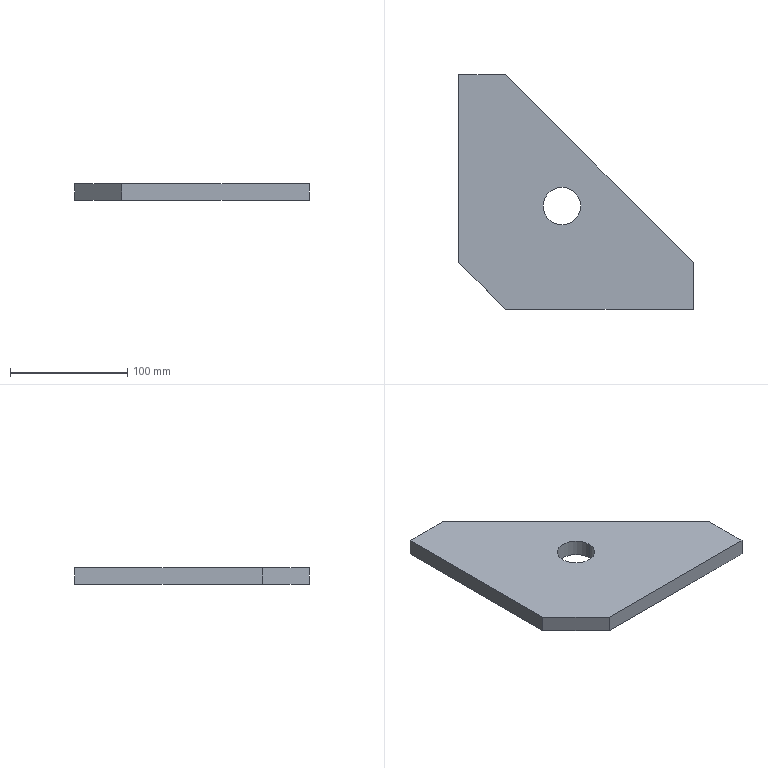Part | SolidWorks | features Extrusion 1 | 1 solid | 10 faces | box 200 x 200 x 14 mm | volume 358341 mm3 | plane 8 | cylinder 2 | commonest cylinder face diameters 32 x2
STEP:
#1=CARTESIAN_POINT('',(72.,-112.,14.));
#2=VERTEX_POINT('',#1);
#3=CARTESIAN_POINT('',(104.,-112.,14.));
#4=VERTEX_POINT('',#3);
#5=CARTESIAN_POINT('',(88.,-112.,14.));
#6=DIRECTION('',(0.,0.,1.));
#7=DIRECTION('',(1.,0.,0.));
#8=AXIS2_PLACEMENT_3D('',#5,#6,#7);
#9=CIRCLE('',#8,16.);
#10=EDGE_CURVE('',#2,#4,#9,.T.);
#11=ORIENTED_EDGE('',*,*,#10,.T.);
#12=CARTESIAN_POINT('',(104.,-112.,0.));
#13=VERTEX_POINT('',#12);
#14=CARTESIAN_POINT('',(104.,-112.,14.));
#15=DIRECTION('',(0.,0.,-1.));
#16=VECTOR('',#15,1000.);
#17=LINE('',#14,#16);
#18=EDGE_CURVE('',#4,#13,#17,.T.);
#19=ORIENTED_EDGE('',*,*,#18,.T.);
#20=CARTESIAN_POINT('',(72.,-112.,0.));
#21=VERTEX_POINT('',#20);
#22=CARTESIAN_POINT('',(88.,-112.,0.));
#23=DIRECTION('',(0.,0.,1.));
#24=DIRECTION('',(1.,0.,0.));
#25=AXIS2_PLACEMENT_3D('',#22,#23,#24);
#26=CIRCLE('',#25,16.);
#27=EDGE_CURVE('',#21,#13,#26,.T.);
#28=ORIENTED_EDGE('',*,*,#27,.F.);
#29=CARTESIAN_POINT('',(72.,-112.,14.));
#30=DIRECTION('',(0.,0.,-1.));
#31=VECTOR('',#30,1000.);
#32=LINE('',#29,#31);
#33=EDGE_CURVE('',#2,#21,#32,.T.);
#34=ORIENTED_EDGE('',*,*,#33,.F.);
#35=EDGE_LOOP('',(#11,#19,#28,#34));
#36=FACE_OUTER_BOUND('',#35,.T.);
#37=CARTESIAN_POINT('',(88.,-112.,14.));
#38=DIRECTION('',(0.,0.,-1.));
#39=DIRECTION('',(-1.,0.,0.));
#40=AXIS2_PLACEMENT_3D('',#37,#38,#39);
#41=CYLINDRICAL_SURFACE('',#40,16.);
#42=ADVANCED_FACE('',(#36),#41,.F.);
#43=CARTESIAN_POINT('',(0.,0.,14.));
#44=VERTEX_POINT('',#43);
#45=CARTESIAN_POINT('',(0.,-160.,14.));
#46=VERTEX_POINT('',#45);
#47=CARTESIAN_POINT('',(0.,-160.,14.));
#48=DIRECTION('',(0.,-1.,0.));
#49=VECTOR('',#48,1000.);
#50=LINE('',#47,#49);
#51=EDGE_CURVE('',#44,#46,#50,.T.);
#52=ORIENTED_EDGE('',*,*,#51,.T.);
#53=CARTESIAN_POINT('',(40.,-200.,14.));
#54=VERTEX_POINT('',#53);
#55=CARTESIAN_POINT('',(40.,-200.,14.));
#56=DIRECTION('',(0.7071,-0.7071,0.));
#57=VECTOR('',#56,1000.);
#58=LINE('',#55,#57);
#59=EDGE_CURVE('',#46,#54,#58,.T.);
#60=ORIENTED_EDGE('',*,*,#59,.T.);
#61=CARTESIAN_POINT('',(200.,-200.,14.));
#62=VERTEX_POINT('',#61);
#63=CARTESIAN_POINT('',(200.,-200.,14.));
#64=DIRECTION('',(1.,0.,0.));
#65=VECTOR('',#64,1000.);
#66=LINE('',#63,#65);
#67=EDGE_CURVE('',#54,#62,#66,.T.);
#68=ORIENTED_EDGE('',*,*,#67,.T.);
#69=CARTESIAN_POINT('',(200.,-160.,14.));
#70=VERTEX_POINT('',#69);
#71=CARTESIAN_POINT('',(200.,-160.,14.));
#72=DIRECTION('',(0.,1.,0.));
#73=VECTOR('',#72,1000.);
#74=LINE('',#71,#73);
#75=EDGE_CURVE('',#62,#70,#74,.T.);
#76=ORIENTED_EDGE('',*,*,#75,.T.);
#77=CARTESIAN_POINT('',(40.,0.,14.));
#78=VERTEX_POINT('',#77);
#79=CARTESIAN_POINT('',(40.,0.,14.));
#80=DIRECTION('',(-0.7071,0.7071,0.));
#81=VECTOR('',#80,1000.);
#82=LINE('',#79,#81);
#83=EDGE_CURVE('',#70,#78,#82,.T.);
#84=ORIENTED_EDGE('',*,*,#83,.T.);
#85=CARTESIAN_POINT('',(0.,0.,14.));
#86=DIRECTION('',(-1.,0.,0.));
#87=VECTOR('',#86,1000.);
#88=LINE('',#85,#87);
#89=EDGE_CURVE('',#78,#44,#88,.T.);
#90=ORIENTED_EDGE('',*,*,#89,.T.);
#91=EDGE_LOOP('',(#52,#60,#68,#76,#84,#90));
#92=FACE_OUTER_BOUND('',#91,.T.);
#93=ORIENTED_EDGE('',*,*,#10,.F.);
#94=CARTESIAN_POINT('',(88.,-112.,14.));
#95=DIRECTION('',(0.,0.,1.));
#96=DIRECTION('',(1.,0.,0.));
#97=AXIS2_PLACEMENT_3D('',#94,#95,#96);
#98=CIRCLE('',#97,16.);
#99=EDGE_CURVE('',#4,#2,#98,.T.);
#100=ORIENTED_EDGE('',*,*,#99,.F.);
#101=EDGE_LOOP('',(#93,#100));
#102=FACE_BOUND('',#101,.T.);
#103=CARTESIAN_POINT('',(0.,0.,14.));
#104=DIRECTION('',(0.,0.,-1.));
#105=DIRECTION('',(-1.,0.,0.));
#106=AXIS2_PLACEMENT_3D('',#103,#104,#105);
#107=PLANE('',#106);
#108=ADVANCED_FACE('',(#92,#102),#107,.F.);
#109=CARTESIAN_POINT('',(0.,0.,0.));
#110=VERTEX_POINT('',#109);
#111=CARTESIAN_POINT('',(0.,-160.,0.));
#112=VERTEX_POINT('',#111);
#113=CARTESIAN_POINT('',(0.,-160.,0.));
#114=DIRECTION('',(0.,-1.,0.));
#115=VECTOR('',#114,1000.);
#116=LINE('',#113,#115);
#117=EDGE_CURVE('',#110,#112,#116,.T.);
#118=ORIENTED_EDGE('',*,*,#117,.F.);
#119=CARTESIAN_POINT('',(40.,0.,0.));
#120=VERTEX_POINT('',#119);
#121=CARTESIAN_POINT('',(0.,0.,0.));
#122=DIRECTION('',(-1.,0.,0.));
#123=VECTOR('',#122,1000.);
#124=LINE('',#121,#123);
#125=EDGE_CURVE('',#120,#110,#124,.T.);
#126=ORIENTED_EDGE('',*,*,#125,.F.);
#127=CARTESIAN_POINT('',(200.,-160.,0.));
#128=VERTEX_POINT('',#127);
#129=CARTESIAN_POINT('',(40.,0.,0.));
#130=DIRECTION('',(-0.7071,0.7071,0.));
#131=VECTOR('',#130,1000.);
#132=LINE('',#129,#131);
#133=EDGE_CURVE('',#128,#120,#132,.T.);
#134=ORIENTED_EDGE('',*,*,#133,.F.);
#135=CARTESIAN_POINT('',(200.,-200.,0.));
#136=VERTEX_POINT('',#135);
#137=CARTESIAN_POINT('',(200.,-160.,0.));
#138=DIRECTION('',(0.,1.,0.));
#139=VECTOR('',#138,1000.);
#140=LINE('',#137,#139);
#141=EDGE_CURVE('',#136,#128,#140,.T.);
#142=ORIENTED_EDGE('',*,*,#141,.F.);
#143=CARTESIAN_POINT('',(40.,-200.,0.));
#144=VERTEX_POINT('',#143);
#145=CARTESIAN_POINT('',(200.,-200.,0.));
#146=DIRECTION('',(1.,0.,0.));
#147=VECTOR('',#146,1000.);
#148=LINE('',#145,#147);
#149=EDGE_CURVE('',#144,#136,#148,.T.);
#150=ORIENTED_EDGE('',*,*,#149,.F.);
#151=CARTESIAN_POINT('',(40.,-200.,0.));
#152=DIRECTION('',(0.7071,-0.7071,0.));
#153=VECTOR('',#152,1000.);
#154=LINE('',#151,#153);
#155=EDGE_CURVE('',#112,#144,#154,.T.);
#156=ORIENTED_EDGE('',*,*,#155,.F.);
#157=EDGE_LOOP('',(#118,#126,#134,#142,#150,#156));
#158=FACE_OUTER_BOUND('',#157,.T.);
#159=ORIENTED_EDGE('',*,*,#27,.T.);
#160=CARTESIAN_POINT('',(88.,-112.,0.));
#161=DIRECTION('',(0.,0.,1.));
#162=DIRECTION('',(1.,0.,0.));
#163=AXIS2_PLACEMENT_3D('',#160,#161,#162);
#164=CIRCLE('',#163,16.);
#165=EDGE_CURVE('',#13,#21,#164,.T.);
#166=ORIENTED_EDGE('',*,*,#165,.T.);
#167=EDGE_LOOP('',(#159,#166));
#168=FACE_BOUND('',#167,.T.);
#169=CARTESIAN_POINT('',(0.,0.,0.));
#170=DIRECTION('',(0.,0.,-1.));
#171=DIRECTION('',(-1.,0.,0.));
#172=AXIS2_PLACEMENT_3D('',#169,#170,#171);
#173=PLANE('',#172);
#174=ADVANCED_FACE('',(#158,#168),#173,.T.);
#175=ORIENTED_EDGE('',*,*,#117,.T.);
#176=CARTESIAN_POINT('',(0.,-160.,14.));
#177=DIRECTION('',(0.,0.,-1.));
#178=VECTOR('',#177,1000.);
#179=LINE('',#176,#178);
#180=EDGE_CURVE('',#46,#112,#179,.T.);
#181=ORIENTED_EDGE('',*,*,#180,.F.);
#182=ORIENTED_EDGE('',*,*,#51,.F.);
#183=CARTESIAN_POINT('',(0.,0.,14.));
#184=DIRECTION('',(0.,0.,-1.));
#185=VECTOR('',#184,1000.);
#186=LINE('',#183,#185);
#187=EDGE_CURVE('',#44,#110,#186,.T.);
#188=ORIENTED_EDGE('',*,*,#187,.T.);
#189=EDGE_LOOP('',(#175,#181,#182,#188));
#190=FACE_OUTER_BOUND('',#189,.T.);
#191=CARTESIAN_POINT('',(0.,-160.,14.));
#192=DIRECTION('',(1.,0.,0.));
#193=DIRECTION('',(0.,1.,0.));
#194=AXIS2_PLACEMENT_3D('',#191,#192,#193);
#195=PLANE('',#194);
#196=ADVANCED_FACE('',(#190),#195,.F.);
#197=ORIENTED_EDGE('',*,*,#155,.T.);
#198=CARTESIAN_POINT('',(40.,-200.,14.));
#199=DIRECTION('',(0.,0.,-1.));
#200=VECTOR('',#199,1000.);
#201=LINE('',#198,#200);
#202=EDGE_CURVE('',#54,#144,#201,.T.);
#203=ORIENTED_EDGE('',*,*,#202,.F.);
#204=ORIENTED_EDGE('',*,*,#59,.F.);
#205=ORIENTED_EDGE('',*,*,#180,.T.);
#206=EDGE_LOOP('',(#197,#203,#204,#205));
#207=FACE_OUTER_BOUND('',#206,.T.);
#208=CARTESIAN_POINT('',(40.,-200.,14.));
#209=DIRECTION('',(0.7071,0.7071,0.));
#210=DIRECTION('',(-0.7071,0.7071,0.));
#211=AXIS2_PLACEMENT_3D('',#208,#209,#210);
#212=PLANE('',#211);
#213=ADVANCED_FACE('',(#207),#212,.F.);
#214=ORIENTED_EDGE('',*,*,#149,.T.);
#215=CARTESIAN_POINT('',(200.,-200.,14.));
#216=DIRECTION('',(0.,0.,-1.));
#217=VECTOR('',#216,1000.);
#218=LINE('',#215,#217);
#219=EDGE_CURVE('',#62,#136,#218,.T.);
#220=ORIENTED_EDGE('',*,*,#219,.F.);
#221=ORIENTED_EDGE('',*,*,#67,.F.);
#222=ORIENTED_EDGE('',*,*,#202,.T.);
#223=EDGE_LOOP('',(#214,#220,#221,#222));
#224=FACE_OUTER_BOUND('',#223,.T.);
#225=CARTESIAN_POINT('',(200.,-200.,14.));
#226=DIRECTION('',(0.,1.,0.));
#227=DIRECTION('',(-1.,0.,0.));
#228=AXIS2_PLACEMENT_3D('',#225,#226,#227);
#229=PLANE('',#228);
#230=ADVANCED_FACE('',(#224),#229,.F.);
#231=ORIENTED_EDGE('',*,*,#141,.T.);
#232=CARTESIAN_POINT('',(200.,-160.,14.));
#233=DIRECTION('',(0.,0.,-1.));
#234=VECTOR('',#233,1000.);
#235=LINE('',#232,#234);
#236=EDGE_CURVE('',#70,#128,#235,.T.);
#237=ORIENTED_EDGE('',*,*,#236,.F.);
#238=ORIENTED_EDGE('',*,*,#75,.F.);
#239=ORIENTED_EDGE('',*,*,#219,.T.);
#240=EDGE_LOOP('',(#231,#237,#238,#239));
#241=FACE_OUTER_BOUND('',#240,.T.);
#242=CARTESIAN_POINT('',(200.,-160.,14.));
#243=DIRECTION('',(-1.,0.,0.));
#244=DIRECTION('',(0.,0.,1.));
#245=AXIS2_PLACEMENT_3D('',#242,#243,#244);
#246=PLANE('',#245);
#247=ADVANCED_FACE('',(#241),#246,.F.);
#248=ORIENTED_EDGE('',*,*,#133,.T.);
#249=CARTESIAN_POINT('',(40.,0.,14.));
#250=DIRECTION('',(0.,0.,-1.));
#251=VECTOR('',#250,1000.);
#252=LINE('',#249,#251);
#253=EDGE_CURVE('',#78,#120,#252,.T.);
#254=ORIENTED_EDGE('',*,*,#253,.F.);
#255=ORIENTED_EDGE('',*,*,#83,.F.);
#256=ORIENTED_EDGE('',*,*,#236,.T.);
#257=EDGE_LOOP('',(#248,#254,#255,#256));
#258=FACE_OUTER_BOUND('',#257,.T.);
#259=CARTESIAN_POINT('',(40.,0.,14.));
#260=DIRECTION('',(-0.7071,-0.7071,0.));
#261=DIRECTION('',(0.7071,-0.7071,0.));
#262=AXIS2_PLACEMENT_3D('',#259,#260,#261);
#263=PLANE('',#262);
#264=ADVANCED_FACE('',(#258),#263,.F.);
#265=ORIENTED_EDGE('',*,*,#125,.T.);
#266=ORIENTED_EDGE('',*,*,#187,.F.);
#267=ORIENTED_EDGE('',*,*,#89,.F.);
#268=ORIENTED_EDGE('',*,*,#253,.T.);
#269=EDGE_LOOP('',(#265,#266,#267,#268));
#270=FACE_OUTER_BOUND('',#269,.T.);
#271=CARTESIAN_POINT('',(0.,0.,14.));
#272=DIRECTION('',(0.,-1.,0.));
#273=DIRECTION('',(0.,0.,-1.));
#274=AXIS2_PLACEMENT_3D('',#271,#272,#273);
#275=PLANE('',#274);
#276=ADVANCED_FACE('',(#270),#275,.F.);
#277=ORIENTED_EDGE('',*,*,#18,.F.);
#278=ORIENTED_EDGE('',*,*,#99,.T.);
#279=ORIENTED_EDGE('',*,*,#33,.T.);
#280=ORIENTED_EDGE('',*,*,#165,.F.);
#281=EDGE_LOOP('',(#277,#278,#279,#280));
#282=FACE_OUTER_BOUND('',#281,.T.);
#283=CARTESIAN_POINT('',(88.,-112.,14.));
#284=DIRECTION('',(0.,0.,-1.));
#285=DIRECTION('',(-1.,0.,0.));
#286=AXIS2_PLACEMENT_3D('',#283,#284,#285);
#287=CYLINDRICAL_SURFACE('',#286,16.);
#288=ADVANCED_FACE('',(#282),#287,.F.);
#289=CLOSED_SHELL('',(#42,#108,#174,#196,#213,#230,#247,#264,#276,#288));
#290=MANIFOLD_SOLID_BREP('',#289);
#291=CARTESIAN_POINT('',(0.,0.,0.));
#292=DIRECTION('',(0.,0.,1.));
#293=DIRECTION('',(1.,0.,0.));
#294=AXIS2_PLACEMENT_3D('',#291,#292,#293);
#295=(LENGTH_UNIT()NAMED_UNIT(*)SI_UNIT(.MILLI.,.METRE.));
#296=UNCERTAINTY_MEASURE_WITH_UNIT(LENGTH_MEASURE(0.00001),#295,'','');
#297=(NAMED_UNIT(*)PLANE_ANGLE_UNIT()SI_UNIT($,.RADIAN.));
#298=(NAMED_UNIT(*)SI_UNIT($,.STERADIAN.)SOLID_ANGLE_UNIT());
#299=(GEOMETRIC_REPRESENTATION_CONTEXT(3)GLOBAL_UNCERTAINTY_ASSIGNED_CONTEXT((#296))GLOBAL_UNIT_ASSIGNED_CONTEXT((#295,#297,#298))REPRESENTATION_CONTEXT('',''));
#300=ADVANCED_BREP_SHAPE_REPRESENTATION('',(#290,#294),#299);